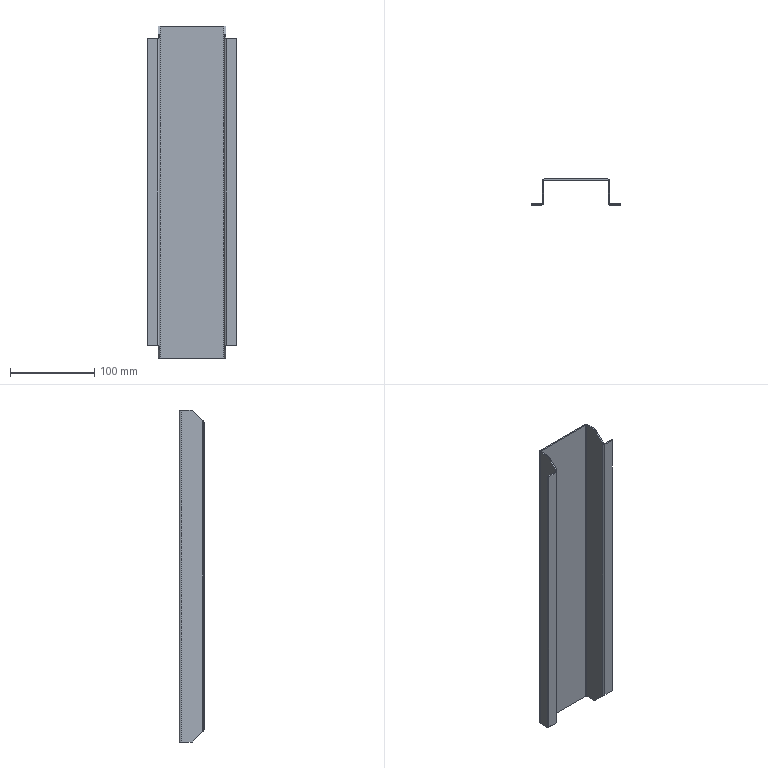Part | SolidWorks | features FlatPattern 1, ICE 1, SMBaseFlange 1, SheetMetal 1 | 1 solid | 42 faces | box 107 x 30.5 x 395 mm | volume 94156 mm3 | plane 30 | cylinder 8 | spline 4 | commonest cylinder face diameters 2 x4 5 x4
STEP:
#1=CARTESIAN_POINT('',(65.477,14.708,15.));
#2=VERTEX_POINT('',#1);
#3=CARTESIAN_POINT('',(52.977,14.708,15.));
#4=VERTEX_POINT('',#3);
#5=CARTESIAN_POINT('',(165.477,14.708,15.));
#6=DIRECTION('',(-1.,0.,0.));
#7=VECTOR('',#6,1000.);
#8=LINE('',#5,#7);
#9=EDGE_CURVE('',#2,#4,#8,.T.);
#10=ORIENTED_EDGE('',*,*,#9,.F.);
#11=CARTESIAN_POINT('',(65.477,14.708,380.));
#12=VERTEX_POINT('',#11);
#13=CARTESIAN_POINT('',(65.477,14.708,395.));
#14=DIRECTION('',(0.,0.,-1.));
#15=VECTOR('',#14,1000.);
#16=LINE('',#13,#15);
#17=EDGE_CURVE('',#12,#2,#16,.T.);
#18=ORIENTED_EDGE('',*,*,#17,.F.);
#19=CARTESIAN_POINT('',(52.977,14.708,380.));
#20=VERTEX_POINT('',#19);
#21=CARTESIAN_POINT('',(165.477,14.708,380.));
#22=DIRECTION('',(-1.,0.,0.));
#23=VECTOR('',#22,1000.);
#24=LINE('',#21,#23);
#25=EDGE_CURVE('',#12,#20,#24,.T.);
#26=ORIENTED_EDGE('',*,*,#25,.T.);
#27=CARTESIAN_POINT('',(52.977,14.708,395.));
#28=DIRECTION('',(0.,0.,-1.));
#29=VECTOR('',#28,1000.);
#30=LINE('',#27,#29);
#31=EDGE_CURVE('',#20,#4,#30,.T.);
#32=ORIENTED_EDGE('',*,*,#31,.T.);
#33=EDGE_LOOP('',(#10,#18,#26,#32));
#34=FACE_OUTER_BOUND('',#33,.T.);
#35=CARTESIAN_POINT('',(51.977,14.708,395.));
#36=DIRECTION('',(0.,1.,0.));
#37=DIRECTION('',(0.,0.,1.));
#38=AXIS2_PLACEMENT_3D('',#35,#36,#37);
#39=PLANE('',#38);
#40=ADVANCED_FACE('',(#34),#39,.F.);
#41=ORIENTED_EDGE('',*,*,#17,.T.);
#42=CARTESIAN_POINT('',(65.477,16.208,15.));
#43=VERTEX_POINT('',#42);
#44=CARTESIAN_POINT('',(65.477,14.708,15.));
#45=DIRECTION('',(0.,1.,0.));
#46=VECTOR('',#45,1000.);
#47=LINE('',#44,#46);
#48=EDGE_CURVE('',#2,#43,#47,.T.);
#49=ORIENTED_EDGE('',*,*,#48,.T.);
#50=CARTESIAN_POINT('',(65.477,16.208,380.));
#51=VERTEX_POINT('',#50);
#52=CARTESIAN_POINT('',(65.477,16.208,395.));
#53=DIRECTION('',(0.,0.,-1.));
#54=VECTOR('',#53,1000.);
#55=LINE('',#52,#54);
#56=EDGE_CURVE('',#51,#43,#55,.T.);
#57=ORIENTED_EDGE('',*,*,#56,.F.);
#58=CARTESIAN_POINT('',(65.477,14.708,380.));
#59=DIRECTION('',(0.,1.,0.));
#60=VECTOR('',#59,1000.);
#61=LINE('',#58,#60);
#62=EDGE_CURVE('',#12,#51,#61,.T.);
#63=ORIENTED_EDGE('',*,*,#62,.F.);
#64=EDGE_LOOP('',(#41,#49,#57,#63));
#65=FACE_OUTER_BOUND('',#64,.T.);
#66=CARTESIAN_POINT('',(65.477,16.208,395.));
#67=DIRECTION('',(1.,0.,0.));
#68=DIRECTION('',(0.,0.,-1.));
#69=AXIS2_PLACEMENT_3D('',#66,#67,#68);
#70=PLANE('',#69);
#71=ADVANCED_FACE('',(#65),#70,.T.);
#72=ORIENTED_EDGE('',*,*,#56,.T.);
#73=CARTESIAN_POINT('',(52.977,16.208,15.));
#74=VERTEX_POINT('',#73);
#75=CARTESIAN_POINT('',(51.977,16.208,15.));
#76=DIRECTION('',(-1.,0.,0.));
#77=VECTOR('',#76,1000.);
#78=LINE('',#75,#77);
#79=EDGE_CURVE('',#43,#74,#78,.T.);
#80=ORIENTED_EDGE('',*,*,#79,.T.);
#81=CARTESIAN_POINT('',(52.977,16.208,380.));
#82=VERTEX_POINT('',#81);
#83=CARTESIAN_POINT('',(52.977,16.208,395.));
#84=DIRECTION('',(0.,0.,-1.));
#85=VECTOR('',#84,1000.);
#86=LINE('',#83,#85);
#87=EDGE_CURVE('',#82,#74,#86,.T.);
#88=ORIENTED_EDGE('',*,*,#87,.F.);
#89=CARTESIAN_POINT('',(51.977,16.208,380.));
#90=DIRECTION('',(-1.,0.,0.));
#91=VECTOR('',#90,1000.);
#92=LINE('',#89,#91);
#93=EDGE_CURVE('',#51,#82,#92,.T.);
#94=ORIENTED_EDGE('',*,*,#93,.F.);
#95=EDGE_LOOP('',(#72,#80,#88,#94));
#96=FACE_OUTER_BOUND('',#95,.T.);
#97=CARTESIAN_POINT('',(51.977,16.208,395.));
#98=DIRECTION('',(0.,1.,0.));
#99=DIRECTION('',(0.,0.,1.));
#100=AXIS2_PLACEMENT_3D('',#97,#98,#99);
#101=PLANE('',#100);
#102=ADVANCED_FACE('',(#96),#101,.T.);
#103=ORIENTED_EDGE('',*,*,#87,.T.);
#104=CARTESIAN_POINT('',(51.977,17.208,12.5));
#105=VERTEX_POINT('',#104);
#106=CARTESIAN_POINT('',(51.977,17.208,12.5));
#107=CARTESIAN_POINT('',(51.977,16.623,13.964));
#108=CARTESIAN_POINT('',(52.391,16.208,15.));
#109=CARTESIAN_POINT('',(52.977,16.208,15.));
#110=(BOUNDED_CURVE()B_SPLINE_CURVE(3,(#106,#107,#108,#109),.UNSPECIFIED.,.F.,.F.)B_SPLINE_CURVE_WITH_KNOTS((4,4),(1.571,3.142),.UNSPECIFIED.)CURVE()GEOMETRIC_REPRESENTATION_ITEM()RATIONAL_B_SPLINE_CURVE((1.,0.8047,0.8047,1.))REPRESENTATION_ITEM(''));
#111=EDGE_CURVE('',#105,#74,#110,.T.);
#112=ORIENTED_EDGE('',*,*,#111,.F.);
#113=CARTESIAN_POINT('',(51.977,17.208,382.5));
#114=VERTEX_POINT('',#113);
#115=CARTESIAN_POINT('',(51.977,17.208,395.));
#116=DIRECTION('',(0.,0.,-1.));
#117=VECTOR('',#116,1000.);
#118=LINE('',#115,#117);
#119=EDGE_CURVE('',#114,#105,#118,.T.);
#120=ORIENTED_EDGE('',*,*,#119,.F.);
#121=CARTESIAN_POINT('',(52.977,16.208,380.));
#122=CARTESIAN_POINT('',(52.391,16.208,380.));
#123=CARTESIAN_POINT('',(51.977,16.623,381.036));
#124=CARTESIAN_POINT('',(51.977,17.208,382.5));
#125=(BOUNDED_CURVE()B_SPLINE_CURVE(3,(#121,#122,#123,#124),.UNSPECIFIED.,.F.,.F.)B_SPLINE_CURVE_WITH_KNOTS((4,4),(0.,1.571),.UNSPECIFIED.)CURVE()GEOMETRIC_REPRESENTATION_ITEM()RATIONAL_B_SPLINE_CURVE((1.,0.8047,0.8047,1.))REPRESENTATION_ITEM(''));
#126=EDGE_CURVE('',#82,#114,#125,.T.);
#127=ORIENTED_EDGE('',*,*,#126,.F.);
#128=EDGE_LOOP('',(#103,#112,#120,#127));
#129=FACE_OUTER_BOUND('',#128,.T.);
#130=CARTESIAN_POINT('',(52.977,17.208,395.));
#131=DIRECTION('',(0.,0.,-1.));
#132=DIRECTION('',(-1.,0.,0.));
#133=AXIS2_PLACEMENT_3D('',#130,#131,#132);
#134=CYLINDRICAL_SURFACE('',#133,1.);
#135=ADVANCED_FACE('',(#129),#134,.F.);
#136=ORIENTED_EDGE('',*,*,#119,.T.);
#137=CARTESIAN_POINT('',(51.977,29.708,0.));
#138=VERTEX_POINT('',#137);
#139=CARTESIAN_POINT('',(51.977,-160.042,189.75));
#140=DIRECTION('',(0.,-0.7071,0.7071));
#141=VECTOR('',#140,1000.);
#142=LINE('',#139,#141);
#143=EDGE_CURVE('',#138,#105,#142,.T.);
#144=ORIENTED_EDGE('',*,*,#143,.F.);
#145=CARTESIAN_POINT('',(51.977,42.708,0.));
#146=VERTEX_POINT('',#145);
#147=CARTESIAN_POINT('',(51.977,45.208,0.));
#148=DIRECTION('',(0.,-1.,0.));
#149=VECTOR('',#148,1000.);
#150=LINE('',#147,#149);
#151=EDGE_CURVE('',#146,#138,#150,.T.);
#152=ORIENTED_EDGE('',*,*,#151,.F.);
#153=CARTESIAN_POINT('',(51.977,42.708,395.));
#154=VERTEX_POINT('',#153);
#155=CARTESIAN_POINT('',(51.977,42.708,395.));
#156=DIRECTION('',(0.,0.,-1.));
#157=VECTOR('',#156,1000.);
#158=LINE('',#155,#157);
#159=EDGE_CURVE('',#154,#146,#158,.T.);
#160=ORIENTED_EDGE('',*,*,#159,.F.);
#161=CARTESIAN_POINT('',(51.977,29.708,395.));
#162=VERTEX_POINT('',#161);
#163=CARTESIAN_POINT('',(51.977,45.208,395.));
#164=DIRECTION('',(0.,-1.,0.));
#165=VECTOR('',#164,1000.);
#166=LINE('',#163,#165);
#167=EDGE_CURVE('',#154,#162,#166,.T.);
#168=ORIENTED_EDGE('',*,*,#167,.T.);
#169=CARTESIAN_POINT('',(51.977,37.458,402.75));
#170=DIRECTION('',(0.,0.7071,0.7071));
#171=VECTOR('',#170,1000.);
#172=LINE('',#169,#171);
#173=EDGE_CURVE('',#114,#162,#172,.T.);
#174=ORIENTED_EDGE('',*,*,#173,.F.);
#175=EDGE_LOOP('',(#136,#144,#152,#160,#168,#174));
#176=FACE_OUTER_BOUND('',#175,.T.);
#177=CARTESIAN_POINT('',(51.977,45.208,395.));
#178=DIRECTION('',(1.,0.,0.));
#179=DIRECTION('',(0.,0.,-1.));
#180=AXIS2_PLACEMENT_3D('',#177,#178,#179);
#181=PLANE('',#180);
#182=ADVANCED_FACE('',(#176),#181,.T.);
#183=CARTESIAN_POINT('',(50.477,29.708,0.));
#184=VERTEX_POINT('',#183);
#185=CARTESIAN_POINT('',(50.477,17.208,12.5));
#186=VERTEX_POINT('',#185);
#187=CARTESIAN_POINT('',(50.477,-160.042,189.75));
#188=DIRECTION('',(0.,-0.7071,0.7071));
#189=VECTOR('',#188,1000.);
#190=LINE('',#187,#189);
#191=EDGE_CURVE('',#184,#186,#190,.T.);
#192=ORIENTED_EDGE('',*,*,#191,.T.);
#193=CARTESIAN_POINT('',(50.477,17.208,382.5));
#194=VERTEX_POINT('',#193);
#195=CARTESIAN_POINT('',(50.477,17.208,395.));
#196=DIRECTION('',(0.,0.,-1.));
#197=VECTOR('',#196,1000.);
#198=LINE('',#195,#197);
#199=EDGE_CURVE('',#194,#186,#198,.T.);
#200=ORIENTED_EDGE('',*,*,#199,.F.);
#201=CARTESIAN_POINT('',(50.477,29.708,395.));
#202=VERTEX_POINT('',#201);
#203=CARTESIAN_POINT('',(50.477,37.458,402.75));
#204=DIRECTION('',(0.,0.7071,0.7071));
#205=VECTOR('',#204,1000.);
#206=LINE('',#203,#205);
#207=EDGE_CURVE('',#194,#202,#206,.T.);
#208=ORIENTED_EDGE('',*,*,#207,.T.);
#209=CARTESIAN_POINT('',(50.477,42.708,395.));
#210=VERTEX_POINT('',#209);
#211=CARTESIAN_POINT('',(50.477,45.208,395.));
#212=DIRECTION('',(0.,-1.,0.));
#213=VECTOR('',#212,1000.);
#214=LINE('',#211,#213);
#215=EDGE_CURVE('',#210,#202,#214,.T.);
#216=ORIENTED_EDGE('',*,*,#215,.F.);
#217=CARTESIAN_POINT('',(50.477,42.708,0.));
#218=VERTEX_POINT('',#217);
#219=CARTESIAN_POINT('',(50.477,42.708,395.));
#220=DIRECTION('',(0.,0.,-1.));
#221=VECTOR('',#220,1000.);
#222=LINE('',#219,#221);
#223=EDGE_CURVE('',#210,#218,#222,.T.);
#224=ORIENTED_EDGE('',*,*,#223,.T.);
#225=CARTESIAN_POINT('',(50.477,45.208,0.));
#226=DIRECTION('',(0.,-1.,0.));
#227=VECTOR('',#226,1000.);
#228=LINE('',#225,#227);
#229=EDGE_CURVE('',#218,#184,#228,.T.);
#230=ORIENTED_EDGE('',*,*,#229,.T.);
#231=EDGE_LOOP('',(#192,#200,#208,#216,#224,#230));
#232=FACE_OUTER_BOUND('',#231,.T.);
#233=CARTESIAN_POINT('',(50.477,45.208,395.));
#234=DIRECTION('',(1.,0.,0.));
#235=DIRECTION('',(0.,0.,-1.));
#236=AXIS2_PLACEMENT_3D('',#233,#234,#235);
#237=PLANE('',#236);
#238=ADVANCED_FACE('',(#232),#237,.F.);
#239=CARTESIAN_POINT('',(50.477,17.208,12.5));
#240=CARTESIAN_POINT('',(50.477,15.744,13.964));
#241=CARTESIAN_POINT('',(51.512,14.708,15.));
#242=CARTESIAN_POINT('',(52.977,14.708,15.));
#243=(BOUNDED_CURVE()B_SPLINE_CURVE(3,(#239,#240,#241,#242),.UNSPECIFIED.,.F.,.F.)B_SPLINE_CURVE_WITH_KNOTS((4,4),(1.571,3.142),.UNSPECIFIED.)CURVE()GEOMETRIC_REPRESENTATION_ITEM()RATIONAL_B_SPLINE_CURVE((1.,0.8047,0.8047,1.))REPRESENTATION_ITEM(''));
#244=EDGE_CURVE('',#186,#4,#243,.T.);
#245=ORIENTED_EDGE('',*,*,#244,.T.);
#246=ORIENTED_EDGE('',*,*,#31,.F.);
#247=CARTESIAN_POINT('',(52.977,14.708,380.));
#248=CARTESIAN_POINT('',(51.512,14.708,380.));
#249=CARTESIAN_POINT('',(50.477,15.744,381.036));
#250=CARTESIAN_POINT('',(50.477,17.208,382.5));
#251=(BOUNDED_CURVE()B_SPLINE_CURVE(3,(#247,#248,#249,#250),.UNSPECIFIED.,.F.,.F.)B_SPLINE_CURVE_WITH_KNOTS((4,4),(0.,1.571),.UNSPECIFIED.)CURVE()GEOMETRIC_REPRESENTATION_ITEM()RATIONAL_B_SPLINE_CURVE((1.,0.8047,0.8047,1.))REPRESENTATION_ITEM(''));
#252=EDGE_CURVE('',#20,#194,#251,.T.);
#253=ORIENTED_EDGE('',*,*,#252,.T.);
#254=ORIENTED_EDGE('',*,*,#199,.T.);
#255=EDGE_LOOP('',(#245,#246,#253,#254));
#256=FACE_OUTER_BOUND('',#255,.T.);
#257=CARTESIAN_POINT('',(52.977,17.208,395.));
#258=DIRECTION('',(0.,0.,-1.));
#259=DIRECTION('',(-1.,0.,0.));
#260=AXIS2_PLACEMENT_3D('',#257,#258,#259);
#261=CYLINDRICAL_SURFACE('',#260,2.5);
#262=ADVANCED_FACE('',(#256),#261,.T.);
#263=CARTESIAN_POINT('',(-28.023,29.708,0.));
#264=VERTEX_POINT('',#263);
#265=CARTESIAN_POINT('',(-28.023,42.708,0.));
#266=VERTEX_POINT('',#265);
#267=CARTESIAN_POINT('',(-28.023,16.208,0.));
#268=DIRECTION('',(0.,1.,0.));
#269=VECTOR('',#268,1000.);
#270=LINE('',#267,#269);
#271=EDGE_CURVE('',#264,#266,#270,.T.);
#272=ORIENTED_EDGE('',*,*,#271,.F.);
#273=CARTESIAN_POINT('',(-28.023,17.208,12.5));
#274=VERTEX_POINT('',#273);
#275=CARTESIAN_POINT('',(-28.023,-174.542,204.25));
#276=DIRECTION('',(0.,0.7071,-0.7071));
#277=VECTOR('',#276,1000.);
#278=LINE('',#275,#277);
#279=EDGE_CURVE('',#274,#264,#278,.T.);
#280=ORIENTED_EDGE('',*,*,#279,.F.);
#281=CARTESIAN_POINT('',(-28.023,17.208,382.5));
#282=VERTEX_POINT('',#281);
#283=CARTESIAN_POINT('',(-28.023,17.208,395.));
#284=DIRECTION('',(0.,0.,-1.));
#285=VECTOR('',#284,1000.);
#286=LINE('',#283,#285);
#287=EDGE_CURVE('',#282,#274,#286,.T.);
#288=ORIENTED_EDGE('',*,*,#287,.F.);
#289=CARTESIAN_POINT('',(-28.023,29.708,395.));
#290=VERTEX_POINT('',#289);
#291=CARTESIAN_POINT('',(-28.023,22.958,388.25));
#292=DIRECTION('',(0.,-0.7071,-0.7071));
#293=VECTOR('',#292,1000.);
#294=LINE('',#291,#293);
#295=EDGE_CURVE('',#290,#282,#294,.T.);
#296=ORIENTED_EDGE('',*,*,#295,.F.);
#297=CARTESIAN_POINT('',(-28.023,42.708,395.));
#298=VERTEX_POINT('',#297);
#299=CARTESIAN_POINT('',(-28.023,16.208,395.));
#300=DIRECTION('',(0.,1.,0.));
#301=VECTOR('',#300,1000.);
#302=LINE('',#299,#301);
#303=EDGE_CURVE('',#290,#298,#302,.T.);
#304=ORIENTED_EDGE('',*,*,#303,.T.);
#305=CARTESIAN_POINT('',(-28.023,42.708,395.));
#306=DIRECTION('',(0.,0.,-1.));
#307=VECTOR('',#306,1000.);
#308=LINE('',#305,#307);
#309=EDGE_CURVE('',#298,#266,#308,.T.);
#310=ORIENTED_EDGE('',*,*,#309,.T.);
#311=EDGE_LOOP('',(#272,#280,#288,#296,#304,#310));
#312=FACE_OUTER_BOUND('',#311,.T.);
#313=CARTESIAN_POINT('',(-28.023,16.208,395.));
#314=DIRECTION('',(-1.,0.,0.));
#315=DIRECTION('',(0.,0.,1.));
#316=AXIS2_PLACEMENT_3D('',#313,#314,#315);
#317=PLANE('',#316);
#318=ADVANCED_FACE('',(#312),#317,.T.);
#319=ORIENTED_EDGE('',*,*,#287,.T.);
#320=CARTESIAN_POINT('',(-29.023,16.208,15.));
#321=VERTEX_POINT('',#320);
#322=CARTESIAN_POINT('',(-29.023,16.208,15.));
#323=CARTESIAN_POINT('',(-28.437,16.208,15.));
#324=CARTESIAN_POINT('',(-28.023,16.623,13.964));
#325=CARTESIAN_POINT('',(-28.023,17.208,12.5));
#326=(BOUNDED_CURVE()B_SPLINE_CURVE(3,(#322,#323,#324,#325),.UNSPECIFIED.,.F.,.T.)B_SPLINE_CURVE_WITH_KNOTS((4,4),(3.142,4.712),.UNSPECIFIED.)CURVE()GEOMETRIC_REPRESENTATION_ITEM()RATIONAL_B_SPLINE_CURVE((1.,0.8047,0.8047,1.))REPRESENTATION_ITEM(''));
#327=EDGE_CURVE('',#321,#274,#326,.T.);
#328=ORIENTED_EDGE('',*,*,#327,.F.);
#329=CARTESIAN_POINT('',(-29.023,16.208,380.));
#330=VERTEX_POINT('',#329);
#331=CARTESIAN_POINT('',(-29.023,16.208,395.));
#332=DIRECTION('',(0.,0.,-1.));
#333=VECTOR('',#332,1000.);
#334=LINE('',#331,#333);
#335=EDGE_CURVE('',#330,#321,#334,.T.);
#336=ORIENTED_EDGE('',*,*,#335,.F.);
#337=CARTESIAN_POINT('',(-28.023,17.208,382.5));
#338=CARTESIAN_POINT('',(-28.023,16.623,381.036));
#339=CARTESIAN_POINT('',(-28.437,16.208,380.));
#340=CARTESIAN_POINT('',(-29.023,16.208,380.));
#341=(BOUNDED_CURVE()B_SPLINE_CURVE(3,(#337,#338,#339,#340),.UNSPECIFIED.,.F.,.F.)B_SPLINE_CURVE_WITH_KNOTS((4,4),(4.712,6.283),.UNSPECIFIED.)CURVE()GEOMETRIC_REPRESENTATION_ITEM()RATIONAL_B_SPLINE_CURVE((1.,0.8047,0.8047,1.))REPRESENTATION_ITEM(''));
#342=EDGE_CURVE('',#282,#330,#341,.T.);
#343=ORIENTED_EDGE('',*,*,#342,.F.);
#344=EDGE_LOOP('',(#319,#328,#336,#343));
#345=FACE_OUTER_BOUND('',#344,.T.);
#346=CARTESIAN_POINT('',(-29.023,17.208,395.));
#347=DIRECTION('',(0.,0.,-1.));
#348=DIRECTION('',(-1.,0.,0.));
#349=AXIS2_PLACEMENT_3D('',#346,#347,#348);
#350=CYLINDRICAL_SURFACE('',#349,1.);
#351=ADVANCED_FACE('',(#345),#350,.F.);
#352=ORIENTED_EDGE('',*,*,#335,.T.);
#353=CARTESIAN_POINT('',(-41.523,16.208,15.));
#354=VERTEX_POINT('',#353);
#355=CARTESIAN_POINT('',(-41.523,16.208,15.));
#356=DIRECTION('',(-1.,0.,0.));
#357=VECTOR('',#356,1000.);
#358=LINE('',#355,#357);
#359=EDGE_CURVE('',#321,#354,#358,.T.);
#360=ORIENTED_EDGE('',*,*,#359,.T.);
#361=CARTESIAN_POINT('',(-41.523,16.208,380.));
#362=VERTEX_POINT('',#361);
#363=CARTESIAN_POINT('',(-41.523,16.208,395.));
#364=DIRECTION('',(0.,0.,-1.));
#365=VECTOR('',#364,1000.);
#366=LINE('',#363,#365);
#367=EDGE_CURVE('',#362,#354,#366,.T.);
#368=ORIENTED_EDGE('',*,*,#367,.F.);
#369=CARTESIAN_POINT('',(-41.523,16.208,380.));
#370=DIRECTION('',(-1.,0.,0.));
#371=VECTOR('',#370,1000.);
#372=LINE('',#369,#371);
#373=EDGE_CURVE('',#330,#362,#372,.T.);
#374=ORIENTED_EDGE('',*,*,#373,.F.);
#375=EDGE_LOOP('',(#352,#360,#368,#374));
#376=FACE_OUTER_BOUND('',#375,.T.);
#377=CARTESIAN_POINT('',(-41.523,16.208,395.));
#378=DIRECTION('',(0.,1.,0.));
#379=DIRECTION('',(0.,0.,1.));
#380=AXIS2_PLACEMENT_3D('',#377,#378,#379);
#381=PLANE('',#380);
#382=ADVANCED_FACE('',(#376),#381,.T.);
#383=ORIENTED_EDGE('',*,*,#367,.T.);
#384=CARTESIAN_POINT('',(-41.523,14.708,15.));
#385=VERTEX_POINT('',#384);
#386=CARTESIAN_POINT('',(-41.523,14.708,15.));
#387=DIRECTION('',(0.,1.,0.));
#388=VECTOR('',#387,1000.);
#389=LINE('',#386,#388);
#390=EDGE_CURVE('',#385,#354,#389,.T.);
#391=ORIENTED_EDGE('',*,*,#390,.F.);
#392=CARTESIAN_POINT('',(-41.523,14.708,380.));
#393=VERTEX_POINT('',#392);
#394=CARTESIAN_POINT('',(-41.523,14.708,395.));
#395=DIRECTION('',(0.,0.,-1.));
#396=VECTOR('',#395,1000.);
#397=LINE('',#394,#396);
#398=EDGE_CURVE('',#393,#385,#397,.T.);
#399=ORIENTED_EDGE('',*,*,#398,.F.);
#400=CARTESIAN_POINT('',(-41.523,14.708,380.));
#401=DIRECTION('',(0.,1.,0.));
#402=VECTOR('',#401,1000.);
#403=LINE('',#400,#402);
#404=EDGE_CURVE('',#393,#362,#403,.T.);
#405=ORIENTED_EDGE('',*,*,#404,.T.);
#406=EDGE_LOOP('',(#383,#391,#399,#405));
#407=FACE_OUTER_BOUND('',#406,.T.);
#408=CARTESIAN_POINT('',(-41.523,14.708,395.));
#409=DIRECTION('',(-1.,0.,0.));
#410=DIRECTION('',(0.,0.,1.));
#411=AXIS2_PLACEMENT_3D('',#408,#409,#410);
#412=PLANE('',#411);
#413=ADVANCED_FACE('',(#407),#412,.T.);
#414=CARTESIAN_POINT('',(-29.023,14.708,15.));
#415=VERTEX_POINT('',#414);
#416=CARTESIAN_POINT('',(165.477,14.708,15.));
#417=DIRECTION('',(-1.,0.,0.));
#418=VECTOR('',#417,1000.);
#419=LINE('',#416,#418);
#420=EDGE_CURVE('',#415,#385,#419,.T.);
#421=ORIENTED_EDGE('',*,*,#420,.F.);
#422=CARTESIAN_POINT('',(-29.023,14.708,380.));
#423=VERTEX_POINT('',#422);
#424=CARTESIAN_POINT('',(-29.023,14.708,395.));
#425=DIRECTION('',(0.,0.,-1.));
#426=VECTOR('',#425,1000.);
#427=LINE('',#424,#426);
#428=EDGE_CURVE('',#423,#415,#427,.T.);
#429=ORIENTED_EDGE('',*,*,#428,.F.);
#430=CARTESIAN_POINT('',(165.477,14.708,380.));
#431=DIRECTION('',(-1.,0.,0.));
#432=VECTOR('',#431,1000.);
#433=LINE('',#430,#432);
#434=EDGE_CURVE('',#423,#393,#433,.T.);
#435=ORIENTED_EDGE('',*,*,#434,.T.);
#436=ORIENTED_EDGE('',*,*,#398,.T.);
#437=EDGE_LOOP('',(#421,#429,#435,#436));
#438=FACE_OUTER_BOUND('',#437,.T.);
#439=CARTESIAN_POINT('',(-41.523,14.708,395.));
#440=DIRECTION('',(0.,1.,0.));
#441=DIRECTION('',(0.,0.,1.));
#442=AXIS2_PLACEMENT_3D('',#439,#440,#441);
#443=PLANE('',#442);
#444=ADVANCED_FACE('',(#438),#443,.F.);
#445=CARTESIAN_POINT('',(-26.523,17.208,12.5));
#446=VERTEX_POINT('',#445);
#447=CARTESIAN_POINT('',(-29.023,14.708,15.));
#448=CARTESIAN_POINT('',(-27.559,14.708,15.));
#449=CARTESIAN_POINT('',(-26.523,15.744,13.964));
#450=CARTESIAN_POINT('',(-26.523,17.208,12.5));
#451=(BOUNDED_CURVE()B_SPLINE_CURVE(3,(#447,#448,#449,#450),.UNSPECIFIED.,.F.,.F.)B_SPLINE_CURVE_WITH_KNOTS((4,4),(3.142,4.712),.UNSPECIFIED.)CURVE()GEOMETRIC_REPRESENTATION_ITEM()RATIONAL_B_SPLINE_CURVE((1.,0.8047,0.8047,1.))REPRESENTATION_ITEM(''));
#452=EDGE_CURVE('',#415,#446,#451,.T.);
#453=ORIENTED_EDGE('',*,*,#452,.T.);
#454=CARTESIAN_POINT('',(-26.523,17.208,382.5));
#455=VERTEX_POINT('',#454);
#456=CARTESIAN_POINT('',(-26.523,17.208,395.));
#457=DIRECTION('',(0.,0.,-1.));
#458=VECTOR('',#457,1000.);
#459=LINE('',#456,#458);
#460=EDGE_CURVE('',#455,#446,#459,.T.);
#461=ORIENTED_EDGE('',*,*,#460,.F.);
#462=CARTESIAN_POINT('',(-26.523,17.208,382.5));
#463=CARTESIAN_POINT('',(-26.523,15.744,381.036));
#464=CARTESIAN_POINT('',(-27.559,14.708,380.));
#465=CARTESIAN_POINT('',(-29.023,14.708,380.));
#466=(BOUNDED_CURVE()B_SPLINE_CURVE(3,(#462,#463,#464,#465),.UNSPECIFIED.,.F.,.F.)B_SPLINE_CURVE_WITH_KNOTS((4,4),(4.712,6.283),.UNSPECIFIED.)CURVE()GEOMETRIC_REPRESENTATION_ITEM()RATIONAL_B_SPLINE_CURVE((1.,0.8047,0.8047,1.))REPRESENTATION_ITEM(''));
#467=EDGE_CURVE('',#455,#423,#466,.T.);
#468=ORIENTED_EDGE('',*,*,#467,.T.);
#469=ORIENTED_EDGE('',*,*,#428,.T.);
#470=EDGE_LOOP('',(#453,#461,#468,#469));
#471=FACE_OUTER_BOUND('',#470,.T.);
#472=CARTESIAN_POINT('',(-29.023,17.208,395.));
#473=DIRECTION('',(0.,0.,-1.));
#474=DIRECTION('',(-1.,0.,0.));
#475=AXIS2_PLACEMENT_3D('',#472,#473,#474);
#476=CYLINDRICAL_SURFACE('',#475,2.5);
#477=ADVANCED_FACE('',(#471),#476,.T.);
#478=CARTESIAN_POINT('',(-26.523,29.708,0.));
#479=VERTEX_POINT('',#478);
#480=CARTESIAN_POINT('',(-26.523,-174.542,204.25));
#481=DIRECTION('',(0.,0.7071,-0.7071));
#482=VECTOR('',#481,1000.);
#483=LINE('',#480,#482);
#484=EDGE_CURVE('',#446,#479,#483,.T.);
#485=ORIENTED_EDGE('',*,*,#484,.T.);
#486=CARTESIAN_POINT('',(-26.523,42.708,0.));
#487=VERTEX_POINT('',#486);
#488=CARTESIAN_POINT('',(-26.523,16.208,0.));
#489=DIRECTION('',(0.,1.,0.));
#490=VECTOR('',#489,1000.);
#491=LINE('',#488,#490);
#492=EDGE_CURVE('',#479,#487,#491,.T.);
#493=ORIENTED_EDGE('',*,*,#492,.T.);
#494=CARTESIAN_POINT('',(-26.523,42.708,395.));
#495=VERTEX_POINT('',#494);
#496=CARTESIAN_POINT('',(-26.523,42.708,395.));
#497=DIRECTION('',(0.,0.,-1.));
#498=VECTOR('',#497,1000.);
#499=LINE('',#496,#498);
#500=EDGE_CURVE('',#495,#487,#499,.T.);
#501=ORIENTED_EDGE('',*,*,#500,.F.);
#502=CARTESIAN_POINT('',(-26.523,29.708,395.));
#503=VERTEX_POINT('',#502);
#504=CARTESIAN_POINT('',(-26.523,16.208,395.));
#505=DIRECTION('',(0.,1.,0.));
#506=VECTOR('',#505,1000.);
#507=LINE('',#504,#506);
#508=EDGE_CURVE('',#503,#495,#507,.T.);
#509=ORIENTED_EDGE('',*,*,#508,.F.);
#510=CARTESIAN_POINT('',(-26.523,22.958,388.25));
#511=DIRECTION('',(0.,-0.7071,-0.7071));
#512=VECTOR('',#511,1000.);
#513=LINE('',#510,#512);
#514=EDGE_CURVE('',#503,#455,#513,.T.);
#515=ORIENTED_EDGE('',*,*,#514,.T.);
#516=ORIENTED_EDGE('',*,*,#460,.T.);
#517=EDGE_LOOP('',(#485,#493,#501,#509,#515,#516));
#518=FACE_OUTER_BOUND('',#517,.T.);
#519=CARTESIAN_POINT('',(-26.523,16.208,395.));
#520=DIRECTION('',(-1.,0.,0.));
#521=DIRECTION('',(0.,0.,1.));
#522=AXIS2_PLACEMENT_3D('',#519,#520,#521);
#523=PLANE('',#522);
#524=ADVANCED_FACE('',(#518),#523,.F.);
#525=ORIENTED_EDGE('',*,*,#303,.F.);
#526=CARTESIAN_POINT('',(-28.023,29.708,395.));
#527=DIRECTION('',(1.,0.,0.));
#528=VECTOR('',#527,1000.);
#529=LINE('',#526,#528);
#530=EDGE_CURVE('',#290,#503,#529,.T.);
#531=ORIENTED_EDGE('',*,*,#530,.T.);
#532=ORIENTED_EDGE('',*,*,#508,.T.);
#533=CARTESIAN_POINT('',(-26.523,42.708,395.));
#534=DIRECTION('',(-1.,0.,0.));
#535=VECTOR('',#534,1000.);
#536=LINE('',#533,#535);
#537=EDGE_CURVE('',#495,#298,#536,.T.);
#538=ORIENTED_EDGE('',*,*,#537,.T.);
#539=EDGE_LOOP('',(#525,#531,#532,#538));
#540=FACE_OUTER_BOUND('',#539,.T.);
#541=CARTESIAN_POINT('',(-29.023,14.708,395.));
#542=DIRECTION('',(0.,0.,1.));
#543=DIRECTION('',(1.,0.,0.));
#544=AXIS2_PLACEMENT_3D('',#541,#542,#543);
#545=PLANE('',#544);
#546=ADVANCED_FACE('',(#540),#545,.T.);
#547=CARTESIAN_POINT('',(-25.523,45.208,395.));
#548=VERTEX_POINT('',#547);
#549=CARTESIAN_POINT('',(-25.523,43.708,395.));
#550=VERTEX_POINT('',#549);
#551=CARTESIAN_POINT('',(-25.523,45.208,395.));
#552=DIRECTION('',(0.,-1.,0.));
#553=VECTOR('',#552,1000.);
#554=LINE('',#551,#553);
#555=EDGE_CURVE('',#548,#550,#554,.T.);
#556=ORIENTED_EDGE('',*,*,#555,.F.);
#557=CARTESIAN_POINT('',(-25.523,42.708,395.));
#558=DIRECTION('',(0.,0.,-1.));
#559=DIRECTION('',(1.,0.,0.));
#560=AXIS2_PLACEMENT_3D('',#557,#558,#559);
#561=CIRCLE('',#560,2.5);
#562=EDGE_CURVE('',#298,#548,#561,.T.);
#563=ORIENTED_EDGE('',*,*,#562,.F.);
#564=ORIENTED_EDGE('',*,*,#537,.F.);
#565=CARTESIAN_POINT('',(-25.523,42.708,395.));
#566=DIRECTION('',(0.,0.,-1.));
#567=DIRECTION('',(1.,0.,0.));
#568=AXIS2_PLACEMENT_3D('',#565,#566,#567);
#569=CIRCLE('',#568,1.);
#570=EDGE_CURVE('',#495,#550,#569,.T.);
#571=ORIENTED_EDGE('',*,*,#570,.T.);
#572=EDGE_LOOP('',(#556,#563,#564,#571));
#573=FACE_OUTER_BOUND('',#572,.T.);
#574=CARTESIAN_POINT('',(-25.523,45.208,395.));
#575=DIRECTION('',(0.,0.,1.));
#576=DIRECTION('',(1.,0.,0.));
#577=AXIS2_PLACEMENT_3D('',#574,#575,#576);
#578=PLANE('',#577);
#579=ADVANCED_FACE('',(#573),#578,.T.);
#580=CARTESIAN_POINT('',(49.477,45.208,395.));
#581=VERTEX_POINT('',#580);
#582=CARTESIAN_POINT('',(-28.023,45.208,395.));
#583=DIRECTION('',(1.,0.,0.));
#584=VECTOR('',#583,1000.);
#585=LINE('',#582,#584);
#586=EDGE_CURVE('',#548,#581,#585,.T.);
#587=ORIENTED_EDGE('',*,*,#586,.F.);
#588=ORIENTED_EDGE('',*,*,#555,.T.);
#589=CARTESIAN_POINT('',(49.477,43.708,395.));
#590=VERTEX_POINT('',#589);
#591=CARTESIAN_POINT('',(-28.023,43.708,395.));
#592=DIRECTION('',(1.,0.,0.));
#593=VECTOR('',#592,1000.);
#594=LINE('',#591,#593);
#595=EDGE_CURVE('',#550,#590,#594,.T.);
#596=ORIENTED_EDGE('',*,*,#595,.T.);
#597=CARTESIAN_POINT('',(49.477,43.708,395.));
#598=DIRECTION('',(0.,1.,0.));
#599=VECTOR('',#598,1000.);
#600=LINE('',#597,#599);
#601=EDGE_CURVE('',#590,#581,#600,.T.);
#602=ORIENTED_EDGE('',*,*,#601,.T.);
#603=EDGE_LOOP('',(#587,#588,#596,#602));
#604=FACE_OUTER_BOUND('',#603,.T.);
#605=CARTESIAN_POINT('',(-26.523,42.708,395.));
#606=DIRECTION('',(0.,0.,1.));
#607=DIRECTION('',(1.,0.,0.));
#608=AXIS2_PLACEMENT_3D('',#605,#606,#607);
#609=PLANE('',#608);
#610=ADVANCED_FACE('',(#604),#609,.T.);
#611=CARTESIAN_POINT('',(-28.023,42.708,0.));
#612=DIRECTION('',(1.,0.,0.));
#613=VECTOR('',#612,1000.);
#614=LINE('',#611,#613);
#615=EDGE_CURVE('',#266,#487,#614,.T.);
#616=ORIENTED_EDGE('',*,*,#615,.F.);
#617=CARTESIAN_POINT('',(-25.523,45.208,0.));
#618=VERTEX_POINT('',#617);
#619=CARTESIAN_POINT('',(-25.523,42.708,0.));
#620=DIRECTION('',(0.,0.,-1.));
#621=DIRECTION('',(1.,0.,0.));
#622=AXIS2_PLACEMENT_3D('',#619,#620,#621);
#623=CIRCLE('',#622,2.5);
#624=EDGE_CURVE('',#266,#618,#623,.T.);
#625=ORIENTED_EDGE('',*,*,#624,.T.);
#626=CARTESIAN_POINT('',(-25.523,43.708,0.));
#627=VERTEX_POINT('',#626);
#628=CARTESIAN_POINT('',(-25.523,43.708,0.));
#629=DIRECTION('',(0.,1.,0.));
#630=VECTOR('',#629,1000.);
#631=LINE('',#628,#630);
#632=EDGE_CURVE('',#627,#618,#631,.T.);
#633=ORIENTED_EDGE('',*,*,#632,.F.);
#634=CARTESIAN_POINT('',(-25.523,42.708,0.));
#635=DIRECTION('',(0.,0.,-1.));
#636=DIRECTION('',(1.,0.,0.));
#637=AXIS2_PLACEMENT_3D('',#634,#635,#636);
#638=CIRCLE('',#637,1.);
#639=EDGE_CURVE('',#487,#627,#638,.T.);
#640=ORIENTED_EDGE('',*,*,#639,.F.);
#641=EDGE_LOOP('',(#616,#625,#633,#640));
#642=FACE_OUTER_BOUND('',#641,.T.);
#643=CARTESIAN_POINT('',(-28.023,42.708,0.));
#644=DIRECTION('',(0.,0.,-1.));
#645=DIRECTION('',(-1.,0.,0.));
#646=AXIS2_PLACEMENT_3D('',#643,#644,#645);
#647=PLANE('',#646);
#648=ADVANCED_FACE('',(#642),#647,.T.);
#649=ORIENTED_EDGE('',*,*,#492,.F.);
#650=CARTESIAN_POINT('',(-28.023,29.708,0.));
#651=DIRECTION('',(1.,0.,0.));
#652=VECTOR('',#651,1000.);
#653=LINE('',#650,#652);
#654=EDGE_CURVE('',#264,#479,#653,.T.);
#655=ORIENTED_EDGE('',*,*,#654,.F.);
#656=ORIENTED_EDGE('',*,*,#271,.T.);
#657=ORIENTED_EDGE('',*,*,#615,.T.);
#658=EDGE_LOOP('',(#649,#655,#656,#657));
#659=FACE_OUTER_BOUND('',#658,.T.);
#660=CARTESIAN_POINT('',(-25.523,43.708,0.));
#661=DIRECTION('',(0.,0.,-1.));
#662=DIRECTION('',(-1.,0.,0.));
#663=AXIS2_PLACEMENT_3D('',#660,#661,#662);
#664=PLANE('',#663);
#665=ADVANCED_FACE('',(#659),#664,.T.);
#666=CARTESIAN_POINT('',(51.977,42.708,395.));
#667=DIRECTION('',(-1.,0.,0.));
#668=VECTOR('',#667,1000.);
#669=LINE('',#666,#668);
#670=EDGE_CURVE('',#154,#210,#669,.T.);
#671=ORIENTED_EDGE('',*,*,#670,.F.);
#672=CARTESIAN_POINT('',(49.477,42.708,395.));
#673=DIRECTION('',(0.,0.,-1.));
#674=DIRECTION('',(1.,0.,0.));
#675=AXIS2_PLACEMENT_3D('',#672,#673,#674);
#676=CIRCLE('',#675,2.5);
#677=EDGE_CURVE('',#581,#154,#676,.T.);
#678=ORIENTED_EDGE('',*,*,#677,.F.);
#679=ORIENTED_EDGE('',*,*,#601,.F.);
#680=CARTESIAN_POINT('',(49.477,42.708,395.));
#681=DIRECTION('',(0.,0.,-1.));
#682=DIRECTION('',(1.,0.,0.));
#683=AXIS2_PLACEMENT_3D('',#680,#681,#682);
#684=CIRCLE('',#683,1.);
#685=EDGE_CURVE('',#590,#210,#684,.T.);
#686=ORIENTED_EDGE('',*,*,#685,.T.);
#687=EDGE_LOOP('',(#671,#678,#679,#686));
#688=FACE_OUTER_BOUND('',#687,.T.);
#689=CARTESIAN_POINT('',(51.977,42.708,395.));
#690=DIRECTION('',(0.,0.,1.));
#691=DIRECTION('',(1.,0.,0.));
#692=AXIS2_PLACEMENT_3D('',#689,#690,#691);
#693=PLANE('',#692);
#694=ADVANCED_FACE('',(#688),#693,.T.);
#695=ORIENTED_EDGE('',*,*,#215,.T.);
#696=CARTESIAN_POINT('',(50.477,29.708,395.));
#697=DIRECTION('',(1.,0.,0.));
#698=VECTOR('',#697,1000.);
#699=LINE('',#696,#698);
#700=EDGE_CURVE('',#202,#162,#699,.T.);
#701=ORIENTED_EDGE('',*,*,#700,.T.);
#702=ORIENTED_EDGE('',*,*,#167,.F.);
#703=ORIENTED_EDGE('',*,*,#670,.T.);
#704=EDGE_LOOP('',(#695,#701,#702,#703));
#705=FACE_OUTER_BOUND('',#704,.T.);
#706=CARTESIAN_POINT('',(49.477,43.708,395.));
#707=DIRECTION('',(0.,0.,1.));
#708=DIRECTION('',(1.,0.,0.));
#709=AXIS2_PLACEMENT_3D('',#706,#707,#708);
#710=PLANE('',#709);
#711=ADVANCED_FACE('',(#705),#710,.T.);
#712=CARTESIAN_POINT('',(49.477,45.208,0.));
#713=VERTEX_POINT('',#712);
#714=CARTESIAN_POINT('',(49.477,43.708,0.));
#715=VERTEX_POINT('',#714);
#716=CARTESIAN_POINT('',(49.477,45.208,0.));
#717=DIRECTION('',(0.,-1.,0.));
#718=VECTOR('',#717,1000.);
#719=LINE('',#716,#718);
#720=EDGE_CURVE('',#713,#715,#719,.T.);
#721=ORIENTED_EDGE('',*,*,#720,.F.);
#722=CARTESIAN_POINT('',(49.477,42.708,0.));
#723=DIRECTION('',(0.,0.,-1.));
#724=DIRECTION('',(1.,0.,0.));
#725=AXIS2_PLACEMENT_3D('',#722,#723,#724);
#726=CIRCLE('',#725,2.5);
#727=EDGE_CURVE('',#713,#146,#726,.T.);
#728=ORIENTED_EDGE('',*,*,#727,.T.);
#729=CARTESIAN_POINT('',(50.477,42.708,0.));
#730=DIRECTION('',(1.,0.,0.));
#731=VECTOR('',#730,1000.);
#732=LINE('',#729,#731);
#733=EDGE_CURVE('',#218,#146,#732,.T.);
#734=ORIENTED_EDGE('',*,*,#733,.F.);
#735=CARTESIAN_POINT('',(49.477,42.708,0.));
#736=DIRECTION('',(0.,0.,-1.));
#737=DIRECTION('',(1.,0.,0.));
#738=AXIS2_PLACEMENT_3D('',#735,#736,#737);
#739=CIRCLE('',#738,1.);
#740=EDGE_CURVE('',#715,#218,#739,.T.);
#741=ORIENTED_EDGE('',*,*,#740,.F.);
#742=EDGE_LOOP('',(#721,#728,#734,#741));
#743=FACE_OUTER_BOUND('',#742,.T.);
#744=CARTESIAN_POINT('',(49.477,45.208,0.));
#745=DIRECTION('',(0.,0.,-1.));
#746=DIRECTION('',(-1.,0.,0.));
#747=AXIS2_PLACEMENT_3D('',#744,#745,#746);
#748=PLANE('',#747);
#749=ADVANCED_FACE('',(#743),#748,.T.);
#750=CARTESIAN_POINT('',(-28.023,45.208,0.));
#751=DIRECTION('',(1.,0.,0.));
#752=VECTOR('',#751,1000.);
#753=LINE('',#750,#752);
#754=EDGE_CURVE('',#618,#713,#753,.T.);
#755=ORIENTED_EDGE('',*,*,#754,.T.);
#756=ORIENTED_EDGE('',*,*,#720,.T.);
#757=CARTESIAN_POINT('',(-28.023,43.708,0.));
#758=DIRECTION('',(1.,0.,0.));
#759=VECTOR('',#758,1000.);
#760=LINE('',#757,#759);
#761=EDGE_CURVE('',#627,#715,#760,.T.);
#762=ORIENTED_EDGE('',*,*,#761,.F.);
#763=ORIENTED_EDGE('',*,*,#632,.T.);
#764=EDGE_LOOP('',(#755,#756,#762,#763));
#765=FACE_OUTER_BOUND('',#764,.T.);
#766=CARTESIAN_POINT('',(50.477,42.708,0.));
#767=DIRECTION('',(0.,0.,-1.));
#768=DIRECTION('',(-1.,0.,0.));
#769=AXIS2_PLACEMENT_3D('',#766,#767,#768);
#770=PLANE('',#769);
#771=ADVANCED_FACE('',(#765),#770,.T.);
#772=ORIENTED_EDGE('',*,*,#151,.T.);
#773=CARTESIAN_POINT('',(51.977,29.708,0.));
#774=DIRECTION('',(-1.,0.,0.));
#775=VECTOR('',#774,1000.);
#776=LINE('',#773,#775);
#777=EDGE_CURVE('',#138,#184,#776,.T.);
#778=ORIENTED_EDGE('',*,*,#777,.T.);
#779=ORIENTED_EDGE('',*,*,#229,.F.);
#780=ORIENTED_EDGE('',*,*,#733,.T.);
#781=EDGE_LOOP('',(#772,#778,#779,#780));
#782=FACE_OUTER_BOUND('',#781,.T.);
#783=CARTESIAN_POINT('',(52.977,14.708,0.));
#784=DIRECTION('',(0.,0.,-1.));
#785=DIRECTION('',(-1.,0.,0.));
#786=AXIS2_PLACEMENT_3D('',#783,#784,#785);
#787=PLANE('',#786);
#788=ADVANCED_FACE('',(#782),#787,.T.);
#789=ORIENTED_EDGE('',*,*,#727,.F.);
#790=CARTESIAN_POINT('',(49.477,45.208,395.));
#791=DIRECTION('',(0.,0.,-1.));
#792=VECTOR('',#791,1000.);
#793=LINE('',#790,#792);
#794=EDGE_CURVE('',#581,#713,#793,.T.);
#795=ORIENTED_EDGE('',*,*,#794,.F.);
#796=ORIENTED_EDGE('',*,*,#677,.T.);
#797=ORIENTED_EDGE('',*,*,#159,.T.);
#798=EDGE_LOOP('',(#789,#795,#796,#797));
#799=FACE_OUTER_BOUND('',#798,.T.);
#800=CARTESIAN_POINT('',(49.477,42.708,395.));
#801=DIRECTION('',(0.,0.,-1.));
#802=DIRECTION('',(-1.,0.,0.));
#803=AXIS2_PLACEMENT_3D('',#800,#801,#802);
#804=CYLINDRICAL_SURFACE('',#803,2.5);
#805=ADVANCED_FACE('',(#799),#804,.T.);
#806=ORIENTED_EDGE('',*,*,#754,.F.);
#807=CARTESIAN_POINT('',(-25.523,45.208,395.));
#808=DIRECTION('',(0.,0.,-1.));
#809=VECTOR('',#808,1000.);
#810=LINE('',#807,#809);
#811=EDGE_CURVE('',#548,#618,#810,.T.);
#812=ORIENTED_EDGE('',*,*,#811,.F.);
#813=ORIENTED_EDGE('',*,*,#586,.T.);
#814=ORIENTED_EDGE('',*,*,#794,.T.);
#815=EDGE_LOOP('',(#806,#812,#813,#814));
#816=FACE_OUTER_BOUND('',#815,.T.);
#817=CARTESIAN_POINT('',(-28.023,45.208,395.));
#818=DIRECTION('',(0.,1.,0.));
#819=DIRECTION('',(0.,0.,1.));
#820=AXIS2_PLACEMENT_3D('',#817,#818,#819);
#821=PLANE('',#820);
#822=ADVANCED_FACE('',(#816),#821,.T.);
#823=ORIENTED_EDGE('',*,*,#624,.F.);
#824=ORIENTED_EDGE('',*,*,#309,.F.);
#825=ORIENTED_EDGE('',*,*,#562,.T.);
#826=ORIENTED_EDGE('',*,*,#811,.T.);
#827=EDGE_LOOP('',(#823,#824,#825,#826));
#828=FACE_OUTER_BOUND('',#827,.T.);
#829=CARTESIAN_POINT('',(-25.523,42.708,395.));
#830=DIRECTION('',(0.,0.,-1.));
#831=DIRECTION('',(-1.,0.,0.));
#832=AXIS2_PLACEMENT_3D('',#829,#830,#831);
#833=CYLINDRICAL_SURFACE('',#832,2.5);
#834=ADVANCED_FACE('',(#828),#833,.T.);
#835=ORIENTED_EDGE('',*,*,#639,.T.);
#836=CARTESIAN_POINT('',(-25.523,43.708,395.));
#837=DIRECTION('',(0.,0.,-1.));
#838=VECTOR('',#837,1000.);
#839=LINE('',#836,#838);
#840=EDGE_CURVE('',#550,#627,#839,.T.);
#841=ORIENTED_EDGE('',*,*,#840,.F.);
#842=ORIENTED_EDGE('',*,*,#570,.F.);
#843=ORIENTED_EDGE('',*,*,#500,.T.);
#844=EDGE_LOOP('',(#835,#841,#842,#843));
#845=FACE_OUTER_BOUND('',#844,.T.);
#846=CARTESIAN_POINT('',(-25.523,42.708,395.));
#847=DIRECTION('',(0.,0.,-1.));
#848=DIRECTION('',(-1.,0.,0.));
#849=AXIS2_PLACEMENT_3D('',#846,#847,#848);
#850=CYLINDRICAL_SURFACE('',#849,1.);
#851=ADVANCED_FACE('',(#845),#850,.F.);
#852=ORIENTED_EDGE('',*,*,#761,.T.);
#853=CARTESIAN_POINT('',(49.477,43.708,395.));
#854=DIRECTION('',(0.,0.,-1.));
#855=VECTOR('',#854,1000.);
#856=LINE('',#853,#855);
#857=EDGE_CURVE('',#590,#715,#856,.T.);
#858=ORIENTED_EDGE('',*,*,#857,.F.);
#859=ORIENTED_EDGE('',*,*,#595,.F.);
#860=ORIENTED_EDGE('',*,*,#840,.T.);
#861=EDGE_LOOP('',(#852,#858,#859,#860));
#862=FACE_OUTER_BOUND('',#861,.T.);
#863=CARTESIAN_POINT('',(-28.023,43.708,395.));
#864=DIRECTION('',(0.,1.,0.));
#865=DIRECTION('',(0.,0.,1.));
#866=AXIS2_PLACEMENT_3D('',#863,#864,#865);
#867=PLANE('',#866);
#868=ADVANCED_FACE('',(#862),#867,.F.);
#869=ORIENTED_EDGE('',*,*,#740,.T.);
#870=ORIENTED_EDGE('',*,*,#223,.F.);
#871=ORIENTED_EDGE('',*,*,#685,.F.);
#872=ORIENTED_EDGE('',*,*,#857,.T.);
#873=EDGE_LOOP('',(#869,#870,#871,#872));
#874=FACE_OUTER_BOUND('',#873,.T.);
#875=CARTESIAN_POINT('',(49.477,42.708,395.));
#876=DIRECTION('',(0.,0.,-1.));
#877=DIRECTION('',(-1.,0.,0.));
#878=AXIS2_PLACEMENT_3D('',#875,#876,#877);
#879=CYLINDRICAL_SURFACE('',#878,1.);
#880=ADVANCED_FACE('',(#874),#879,.F.);
#881=ORIENTED_EDGE('',*,*,#295,.T.);
#882=CARTESIAN_POINT('',(-28.023,17.208,382.5));
#883=DIRECTION('',(1.,0.,0.));
#884=VECTOR('',#883,1000.);
#885=LINE('',#882,#884);
#886=EDGE_CURVE('',#282,#455,#885,.T.);
#887=ORIENTED_EDGE('',*,*,#886,.T.);
#888=ORIENTED_EDGE('',*,*,#514,.F.);
#889=ORIENTED_EDGE('',*,*,#530,.F.);
#890=EDGE_LOOP('',(#881,#887,#888,#889));
#891=FACE_OUTER_BOUND('',#890,.T.);
#892=CARTESIAN_POINT('',(-28.023,22.958,388.25));
#893=DIRECTION('',(0.,0.7071,-0.7071));
#894=DIRECTION('',(0.,-0.7071,-0.7071));
#895=AXIS2_PLACEMENT_3D('',#892,#893,#894);
#896=PLANE('',#895);
#897=ADVANCED_FACE('',(#891),#896,.F.);
#898=ORIENTED_EDGE('',*,*,#404,.F.);
#899=ORIENTED_EDGE('',*,*,#434,.F.);
#900=CARTESIAN_POINT('',(-29.023,14.708,380.));
#901=DIRECTION('',(0.,1.,0.));
#902=VECTOR('',#901,1000.);
#903=LINE('',#900,#902);
#904=EDGE_CURVE('',#423,#330,#903,.T.);
#905=ORIENTED_EDGE('',*,*,#904,.T.);
#906=ORIENTED_EDGE('',*,*,#373,.T.);
#907=EDGE_LOOP('',(#898,#899,#905,#906));
#908=FACE_OUTER_BOUND('',#907,.T.);
#909=CARTESIAN_POINT('',(165.477,14.708,380.));
#910=DIRECTION('',(0.,0.,-1.));
#911=DIRECTION('',(-1.,0.,0.));
#912=AXIS2_PLACEMENT_3D('',#909,#910,#911);
#913=PLANE('',#912);
#914=ADVANCED_FACE('',(#908),#913,.F.);
#915=ORIENTED_EDGE('',*,*,#904,.F.);
#916=ORIENTED_EDGE('',*,*,#467,.F.);
#917=ORIENTED_EDGE('',*,*,#886,.F.);
#918=ORIENTED_EDGE('',*,*,#342,.T.);
#919=EDGE_LOOP('',(#915,#916,#917,#918));
#920=FACE_OUTER_BOUND('',#919,.T.);
#921=CARTESIAN_POINT('',(-29.023,16.208,380.));
#922=CARTESIAN_POINT('',(-29.023,15.708,380.));
#923=CARTESIAN_POINT('',(-29.023,15.208,380.));
#924=CARTESIAN_POINT('',(-29.023,14.708,380.));
#925=CARTESIAN_POINT('',(-31.023,16.208,380.));
#926=CARTESIAN_POINT('',(-32.023,15.708,380.));
#927=CARTESIAN_POINT('',(-33.023,15.208,380.));
#928=CARTESIAN_POINT('',(-34.023,14.708,380.));
#929=CARTESIAN_POINT('',(-31.023,18.208,385.));
#930=CARTESIAN_POINT('',(-32.023,18.708,385.));
#931=CARTESIAN_POINT('',(-33.023,19.208,385.));
#932=CARTESIAN_POINT('',(-34.023,19.708,385.));
#933=CARTESIAN_POINT('',(-29.023,18.208,385.));
#934=CARTESIAN_POINT('',(-29.023,18.708,385.));
#935=CARTESIAN_POINT('',(-29.023,19.208,385.));
#936=CARTESIAN_POINT('',(-29.023,19.708,385.));
#937=CARTESIAN_POINT('',(-27.023,18.208,385.));
#938=CARTESIAN_POINT('',(-26.023,18.708,385.));
#939=CARTESIAN_POINT('',(-25.023,19.208,385.));
#940=CARTESIAN_POINT('',(-24.023,19.708,385.));
#941=CARTESIAN_POINT('',(-27.023,16.208,380.));
#942=CARTESIAN_POINT('',(-26.023,15.708,380.));
#943=CARTESIAN_POINT('',(-25.023,15.208,380.));
#944=CARTESIAN_POINT('',(-24.023,14.708,380.));
#945=CARTESIAN_POINT('',(-29.023,16.208,380.));
#946=CARTESIAN_POINT('',(-29.023,15.708,380.));
#947=CARTESIAN_POINT('',(-29.023,15.208,380.));
#948=CARTESIAN_POINT('',(-29.023,14.708,380.));
#949=(BOUNDED_SURFACE()B_SPLINE_SURFACE(3,3,((#921,#922,#923,#924),(#925,#926,#927,#928),(#929,#930,#931,#932),(#933,#934,#935,#936),(#937,#938,#939,#940),(#941,#942,#943,#944),(#945,#946,#947,#948)),.UNSPECIFIED.,.T.,.F.,.T.)B_SPLINE_SURFACE_WITH_KNOTS((4,3,4),(4,4),(0.,0.5,1.),(0.,1.),.UNSPECIFIED.)GEOMETRIC_REPRESENTATION_ITEM()RATIONAL_B_SPLINE_SURFACE(((1.,1.,1.,1.),(0.3333,0.3333,0.3333,0.3333),(0.3333,0.3333,0.3333,0.3333),(1.,1.,1.,1.),(0.3333,0.3333,0.3333,0.3333),(0.3333,0.3333,0.3333,0.3333),(1.,1.,1.,1.)))REPRESENTATION_ITEM('')SURFACE());
#950=ADVANCED_FACE('',(#920),#949,.T.);
#951=ORIENTED_EDGE('',*,*,#279,.T.);
#952=ORIENTED_EDGE('',*,*,#654,.T.);
#953=ORIENTED_EDGE('',*,*,#484,.F.);
#954=CARTESIAN_POINT('',(-28.023,17.208,12.5));
#955=DIRECTION('',(1.,0.,0.));
#956=VECTOR('',#955,1000.);
#957=LINE('',#954,#956);
#958=EDGE_CURVE('',#274,#446,#957,.T.);
#959=ORIENTED_EDGE('',*,*,#958,.F.);
#960=EDGE_LOOP('',(#951,#952,#953,#959));
#961=FACE_OUTER_BOUND('',#960,.T.);
#962=CARTESIAN_POINT('',(-28.023,-174.542,204.25));
#963=DIRECTION('',(0.,0.7071,0.7071));
#964=DIRECTION('',(0.,0.7071,-0.7071));
#965=AXIS2_PLACEMENT_3D('',#962,#963,#964);
#966=PLANE('',#965);
#967=ADVANCED_FACE('',(#961),#966,.F.);
#968=CARTESIAN_POINT('',(-29.023,14.708,15.));
#969=DIRECTION('',(0.,1.,0.));
#970=VECTOR('',#969,1000.);
#971=LINE('',#968,#970);
#972=EDGE_CURVE('',#415,#321,#971,.T.);
#973=ORIENTED_EDGE('',*,*,#972,.F.);
#974=ORIENTED_EDGE('',*,*,#420,.T.);
#975=ORIENTED_EDGE('',*,*,#390,.T.);
#976=ORIENTED_EDGE('',*,*,#359,.F.);
#977=EDGE_LOOP('',(#973,#974,#975,#976));
#978=FACE_OUTER_BOUND('',#977,.T.);
#979=CARTESIAN_POINT('',(165.477,14.708,15.));
#980=DIRECTION('',(0.,0.,-1.));
#981=DIRECTION('',(-1.,0.,0.));
#982=AXIS2_PLACEMENT_3D('',#979,#980,#981);
#983=PLANE('',#982);
#984=ADVANCED_FACE('',(#978),#983,.T.);
#985=ORIENTED_EDGE('',*,*,#958,.T.);
#986=ORIENTED_EDGE('',*,*,#452,.F.);
#987=ORIENTED_EDGE('',*,*,#972,.T.);
#988=ORIENTED_EDGE('',*,*,#327,.T.);
#989=EDGE_LOOP('',(#985,#986,#987,#988));
#990=FACE_OUTER_BOUND('',#989,.T.);
#991=CARTESIAN_POINT('',(-29.023,18.208,10.));
#992=CARTESIAN_POINT('',(-29.023,18.708,10.));
#993=CARTESIAN_POINT('',(-29.023,19.208,10.));
#994=CARTESIAN_POINT('',(-29.023,19.708,10.));
#995=CARTESIAN_POINT('',(-31.023,18.208,10.));
#996=CARTESIAN_POINT('',(-32.023,18.708,10.));
#997=CARTESIAN_POINT('',(-33.023,19.208,10.));
#998=CARTESIAN_POINT('',(-34.023,19.708,10.));
#999=CARTESIAN_POINT('',(-31.023,16.208,15.));
#1000=CARTESIAN_POINT('',(-32.023,15.708,15.));
#1001=CARTESIAN_POINT('',(-33.023,15.208,15.));
#1002=CARTESIAN_POINT('',(-34.023,14.708,15.));
#1003=CARTESIAN_POINT('',(-29.023,16.208,15.));
#1004=CARTESIAN_POINT('',(-29.023,15.708,15.));
#1005=CARTESIAN_POINT('',(-29.023,15.208,15.));
#1006=CARTESIAN_POINT('',(-29.023,14.708,15.));
#1007=CARTESIAN_POINT('',(-27.023,16.208,15.));
#1008=CARTESIAN_POINT('',(-26.023,15.708,15.));
#1009=CARTESIAN_POINT('',(-25.023,15.208,15.));
#1010=CARTESIAN_POINT('',(-24.023,14.708,15.));
#1011=CARTESIAN_POINT('',(-27.023,18.208,10.));
#1012=CARTESIAN_POINT('',(-26.023,18.708,10.));
#1013=CARTESIAN_POINT('',(-25.023,19.208,10.));
#1014=CARTESIAN_POINT('',(-24.023,19.708,10.));
#1015=CARTESIAN_POINT('',(-29.023,18.208,10.));
#1016=CARTESIAN_POINT('',(-29.023,18.708,10.));
#1017=CARTESIAN_POINT('',(-29.023,19.208,10.));
#1018=CARTESIAN_POINT('',(-29.023,19.708,10.));
#1019=(BOUNDED_SURFACE()B_SPLINE_SURFACE(3,3,((#991,#992,#993,#994),(#995,#996,#997,#998),(#999,#1000,#1001,#1002),(#1003,#1004,#1005,#1006),(#1007,#1008,#1009,#1010),(#1011,#1012,#1013,#1014),(#1015,#1016,#1017,#1018)),.UNSPECIFIED.,.T.,.F.,.T.)B_SPLINE_SURFACE_WITH_KNOTS((4,3,4),(4,4),(0.,0.5,1.),(0.,1.),.UNSPECIFIED.)GEOMETRIC_REPRESENTATION_ITEM()RATIONAL_B_SPLINE_SURFACE(((1.,1.,1.,1.),(0.3333,0.3333,0.3333,0.3333),(0.3333,0.3333,0.3333,0.3333),(1.,1.,1.,1.),(0.3333,0.3333,0.3333,0.3333),(0.3333,0.3333,0.3333,0.3333),(1.,1.,1.,1.)))REPRESENTATION_ITEM('')SURFACE());
#1020=ADVANCED_FACE('',(#990),#1019,.T.);
#1021=CARTESIAN_POINT('',(52.977,14.708,380.));
#1022=DIRECTION('',(0.,1.,0.));
#1023=VECTOR('',#1022,1000.);
#1024=LINE('',#1021,#1023);
#1025=EDGE_CURVE('',#20,#82,#1024,.T.);
#1026=ORIENTED_EDGE('',*,*,#1025,.F.);
#1027=ORIENTED_EDGE('',*,*,#25,.F.);
#1028=ORIENTED_EDGE('',*,*,#62,.T.);
#1029=ORIENTED_EDGE('',*,*,#93,.T.);
#1030=EDGE_LOOP('',(#1026,#1027,#1028,#1029));
#1031=FACE_OUTER_BOUND('',#1030,.T.);
#1032=CARTESIAN_POINT('',(165.477,14.708,380.));
#1033=DIRECTION('',(0.,0.,-1.));
#1034=DIRECTION('',(-1.,0.,0.));
#1035=AXIS2_PLACEMENT_3D('',#1032,#1033,#1034);
#1036=PLANE('',#1035);
#1037=ADVANCED_FACE('',(#1031),#1036,.F.);
#1038=ORIENTED_EDGE('',*,*,#700,.F.);
#1039=ORIENTED_EDGE('',*,*,#207,.F.);
#1040=CARTESIAN_POINT('',(50.477,17.208,382.5));
#1041=DIRECTION('',(1.,0.,0.));
#1042=VECTOR('',#1041,1000.);
#1043=LINE('',#1040,#1042);
#1044=EDGE_CURVE('',#194,#114,#1043,.T.);
#1045=ORIENTED_EDGE('',*,*,#1044,.T.);
#1046=ORIENTED_EDGE('',*,*,#173,.T.);
#1047=EDGE_LOOP('',(#1038,#1039,#1045,#1046));
#1048=FACE_OUTER_BOUND('',#1047,.T.);
#1049=CARTESIAN_POINT('',(50.477,37.458,402.75));
#1050=DIRECTION('',(0.,0.7071,-0.7071));
#1051=DIRECTION('',(0.,0.7071,0.7071));
#1052=AXIS2_PLACEMENT_3D('',#1049,#1050,#1051);
#1053=PLANE('',#1052);
#1054=ADVANCED_FACE('',(#1048),#1053,.F.);
#1055=ORIENTED_EDGE('',*,*,#1044,.F.);
#1056=ORIENTED_EDGE('',*,*,#252,.F.);
#1057=ORIENTED_EDGE('',*,*,#1025,.T.);
#1058=ORIENTED_EDGE('',*,*,#126,.T.);
#1059=EDGE_LOOP('',(#1055,#1056,#1057,#1058));
#1060=FACE_OUTER_BOUND('',#1059,.T.);
#1061=CARTESIAN_POINT('',(52.977,16.208,380.));
#1062=CARTESIAN_POINT('',(52.977,15.708,380.));
#1063=CARTESIAN_POINT('',(52.977,15.208,380.));
#1064=CARTESIAN_POINT('',(52.977,14.708,380.));
#1065=CARTESIAN_POINT('',(50.977,16.208,380.));
#1066=CARTESIAN_POINT('',(49.977,15.708,380.));
#1067=CARTESIAN_POINT('',(48.977,15.208,380.));
#1068=CARTESIAN_POINT('',(47.977,14.708,380.));
#1069=CARTESIAN_POINT('',(50.977,18.208,385.));
#1070=CARTESIAN_POINT('',(49.977,18.708,385.));
#1071=CARTESIAN_POINT('',(48.977,19.208,385.));
#1072=CARTESIAN_POINT('',(47.977,19.708,385.));
#1073=CARTESIAN_POINT('',(52.977,18.208,385.));
#1074=CARTESIAN_POINT('',(52.977,18.708,385.));
#1075=CARTESIAN_POINT('',(52.977,19.208,385.));
#1076=CARTESIAN_POINT('',(52.977,19.708,385.));
#1077=CARTESIAN_POINT('',(54.977,18.208,385.));
#1078=CARTESIAN_POINT('',(55.977,18.708,385.));
#1079=CARTESIAN_POINT('',(56.977,19.208,385.));
#1080=CARTESIAN_POINT('',(57.977,19.708,385.));
#1081=CARTESIAN_POINT('',(54.977,16.208,380.));
#1082=CARTESIAN_POINT('',(55.977,15.708,380.));
#1083=CARTESIAN_POINT('',(56.977,15.208,380.));
#1084=CARTESIAN_POINT('',(57.977,14.708,380.));
#1085=CARTESIAN_POINT('',(52.977,16.208,380.));
#1086=CARTESIAN_POINT('',(52.977,15.708,380.));
#1087=CARTESIAN_POINT('',(52.977,15.208,380.));
#1088=CARTESIAN_POINT('',(52.977,14.708,380.));
#1089=(BOUNDED_SURFACE()B_SPLINE_SURFACE(3,3,((#1061,#1062,#1063,#1064),(#1065,#1066,#1067,#1068),(#1069,#1070,#1071,#1072),(#1073,#1074,#1075,#1076),(#1077,#1078,#1079,#1080),(#1081,#1082,#1083,#1084),(#1085,#1086,#1087,#1088)),.UNSPECIFIED.,.T.,.F.,.T.)B_SPLINE_SURFACE_WITH_KNOTS((4,3,4),(4,4),(0.,0.5,1.),(0.,1.),.UNSPECIFIED.)GEOMETRIC_REPRESENTATION_ITEM()RATIONAL_B_SPLINE_SURFACE(((1.,1.,1.,1.),(0.3333,0.3333,0.3333,0.3333),(0.3333,0.3333,0.3333,0.3333),(1.,1.,1.,1.),(0.3333,0.3333,0.3333,0.3333),(0.3333,0.3333,0.3333,0.3333),(1.,1.,1.,1.)))REPRESENTATION_ITEM('')SURFACE());
#1090=ADVANCED_FACE('',(#1060),#1089,.T.);
#1091=ORIENTED_EDGE('',*,*,#48,.F.);
#1092=ORIENTED_EDGE('',*,*,#9,.T.);
#1093=CARTESIAN_POINT('',(52.977,14.708,15.));
#1094=DIRECTION('',(0.,1.,0.));
#1095=VECTOR('',#1094,1000.);
#1096=LINE('',#1093,#1095);
#1097=EDGE_CURVE('',#4,#74,#1096,.T.);
#1098=ORIENTED_EDGE('',*,*,#1097,.T.);
#1099=ORIENTED_EDGE('',*,*,#79,.F.);
#1100=EDGE_LOOP('',(#1091,#1092,#1098,#1099));
#1101=FACE_OUTER_BOUND('',#1100,.T.);
#1102=CARTESIAN_POINT('',(165.477,14.708,15.));
#1103=DIRECTION('',(0.,0.,-1.));
#1104=DIRECTION('',(-1.,0.,0.));
#1105=AXIS2_PLACEMENT_3D('',#1102,#1103,#1104);
#1106=PLANE('',#1105);
#1107=ADVANCED_FACE('',(#1101),#1106,.T.);
#1108=ORIENTED_EDGE('',*,*,#143,.T.);
#1109=CARTESIAN_POINT('',(51.977,17.208,12.5));
#1110=DIRECTION('',(-1.,0.,0.));
#1111=VECTOR('',#1110,1000.);
#1112=LINE('',#1109,#1111);
#1113=EDGE_CURVE('',#105,#186,#1112,.T.);
#1114=ORIENTED_EDGE('',*,*,#1113,.T.);
#1115=ORIENTED_EDGE('',*,*,#191,.F.);
#1116=ORIENTED_EDGE('',*,*,#777,.F.);
#1117=EDGE_LOOP('',(#1108,#1114,#1115,#1116));
#1118=FACE_OUTER_BOUND('',#1117,.T.);
#1119=CARTESIAN_POINT('',(51.977,-160.042,189.75));
#1120=DIRECTION('',(0.,0.7071,0.7071));
#1121=DIRECTION('',(0.,-0.7071,0.7071));
#1122=AXIS2_PLACEMENT_3D('',#1119,#1120,#1121);
#1123=PLANE('',#1122);
#1124=ADVANCED_FACE('',(#1118),#1123,.F.);
#1125=ORIENTED_EDGE('',*,*,#1097,.F.);
#1126=ORIENTED_EDGE('',*,*,#244,.F.);
#1127=ORIENTED_EDGE('',*,*,#1113,.F.);
#1128=ORIENTED_EDGE('',*,*,#111,.T.);
#1129=EDGE_LOOP('',(#1125,#1126,#1127,#1128));
#1130=FACE_OUTER_BOUND('',#1129,.T.);
#1131=CARTESIAN_POINT('',(52.977,18.208,10.));
#1132=CARTESIAN_POINT('',(52.977,18.708,10.));
#1133=CARTESIAN_POINT('',(52.977,19.208,10.));
#1134=CARTESIAN_POINT('',(52.977,19.708,10.));
#1135=CARTESIAN_POINT('',(50.977,18.208,10.));
#1136=CARTESIAN_POINT('',(49.977,18.708,10.));
#1137=CARTESIAN_POINT('',(48.977,19.208,10.));
#1138=CARTESIAN_POINT('',(47.977,19.708,10.));
#1139=CARTESIAN_POINT('',(50.977,16.208,15.));
#1140=CARTESIAN_POINT('',(49.977,15.708,15.));
#1141=CARTESIAN_POINT('',(48.977,15.208,15.));
#1142=CARTESIAN_POINT('',(47.977,14.708,15.));
#1143=CARTESIAN_POINT('',(52.977,16.208,15.));
#1144=CARTESIAN_POINT('',(52.977,15.708,15.));
#1145=CARTESIAN_POINT('',(52.977,15.208,15.));
#1146=CARTESIAN_POINT('',(52.977,14.708,15.));
#1147=CARTESIAN_POINT('',(54.977,16.208,15.));
#1148=CARTESIAN_POINT('',(55.977,15.708,15.));
#1149=CARTESIAN_POINT('',(56.977,15.208,15.));
#1150=CARTESIAN_POINT('',(57.977,14.708,15.));
#1151=CARTESIAN_POINT('',(54.977,18.208,10.));
#1152=CARTESIAN_POINT('',(55.977,18.708,10.));
#1153=CARTESIAN_POINT('',(56.977,19.208,10.));
#1154=CARTESIAN_POINT('',(57.977,19.708,10.));
#1155=CARTESIAN_POINT('',(52.977,18.208,10.));
#1156=CARTESIAN_POINT('',(52.977,18.708,10.));
#1157=CARTESIAN_POINT('',(52.977,19.208,10.));
#1158=CARTESIAN_POINT('',(52.977,19.708,10.));
#1159=(BOUNDED_SURFACE()B_SPLINE_SURFACE(3,3,((#1131,#1132,#1133,#1134),(#1135,#1136,#1137,#1138),(#1139,#1140,#1141,#1142),(#1143,#1144,#1145,#1146),(#1147,#1148,#1149,#1150),(#1151,#1152,#1153,#1154),(#1155,#1156,#1157,#1158)),.UNSPECIFIED.,.T.,.F.,.T.)B_SPLINE_SURFACE_WITH_KNOTS((4,3,4),(4,4),(0.,0.5,1.),(0.,1.),.UNSPECIFIED.)GEOMETRIC_REPRESENTATION_ITEM()RATIONAL_B_SPLINE_SURFACE(((1.,1.,1.,1.),(0.3333,0.3333,0.3333,0.3333),(0.3333,0.3333,0.3333,0.3333),(1.,1.,1.,1.),(0.3333,0.3333,0.3333,0.3333),(0.3333,0.3333,0.3333,0.3333),(1.,1.,1.,1.)))REPRESENTATION_ITEM('')SURFACE());
#1160=ADVANCED_FACE('',(#1130),#1159,.T.);
#1161=CLOSED_SHELL('',(#40,#71,#102,#135,#182,#238,#262,#318,#351,#382,#413,#444,#477,#524,#546,#579,#610,#648,#665,#694,#711,#749,#771,#788,#805,#822,#834,#851,#868,#880,#897,#914,#950,#967,#984,#1020,#1037,#1054,#1090,#1107,#1124,#1160));
#1162=MANIFOLD_SOLID_BREP('',#1161);
#1163=CARTESIAN_POINT('',(0.,0.,0.));
#1164=DIRECTION('',(0.,0.,1.));
#1165=DIRECTION('',(1.,0.,0.));
#1166=AXIS2_PLACEMENT_3D('',#1163,#1164,#1165);
#1167=(LENGTH_UNIT()NAMED_UNIT(*)SI_UNIT(.MILLI.,.METRE.));
#1168=UNCERTAINTY_MEASURE_WITH_UNIT(LENGTH_MEASURE(0.00001),#1167,'','');
#1169=(NAMED_UNIT(*)PLANE_ANGLE_UNIT()SI_UNIT($,.RADIAN.));
#1170=(NAMED_UNIT(*)SI_UNIT($,.STERADIAN.)SOLID_ANGLE_UNIT());
#1171=(GEOMETRIC_REPRESENTATION_CONTEXT(3)GLOBAL_UNCERTAINTY_ASSIGNED_CONTEXT((#1168))GLOBAL_UNIT_ASSIGNED_CONTEXT((#1167,#1169,#1170))REPRESENTATION_CONTEXT('',''));
#1172=ADVANCED_BREP_SHAPE_REPRESENTATION('',(#1162,#1166),#1171);